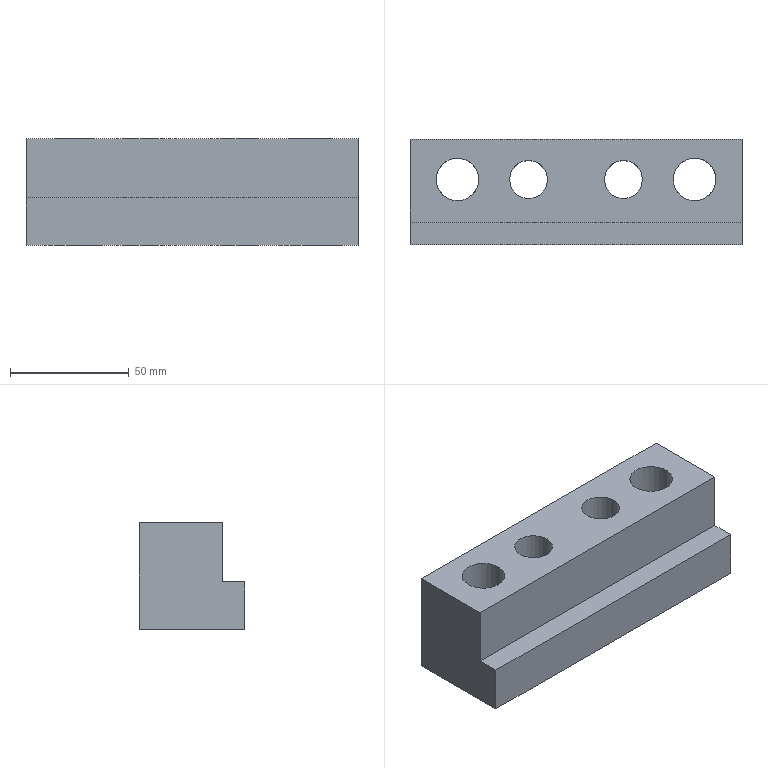Part | STEP file | solid 231 | 1 solid | 16 faces | box 140 x 44.5 x 45 mm | volume 196703 mm3 | plane 10 | cylinder 6 | commonest cylinder face diameters 16 x2 18 x2 26 x2